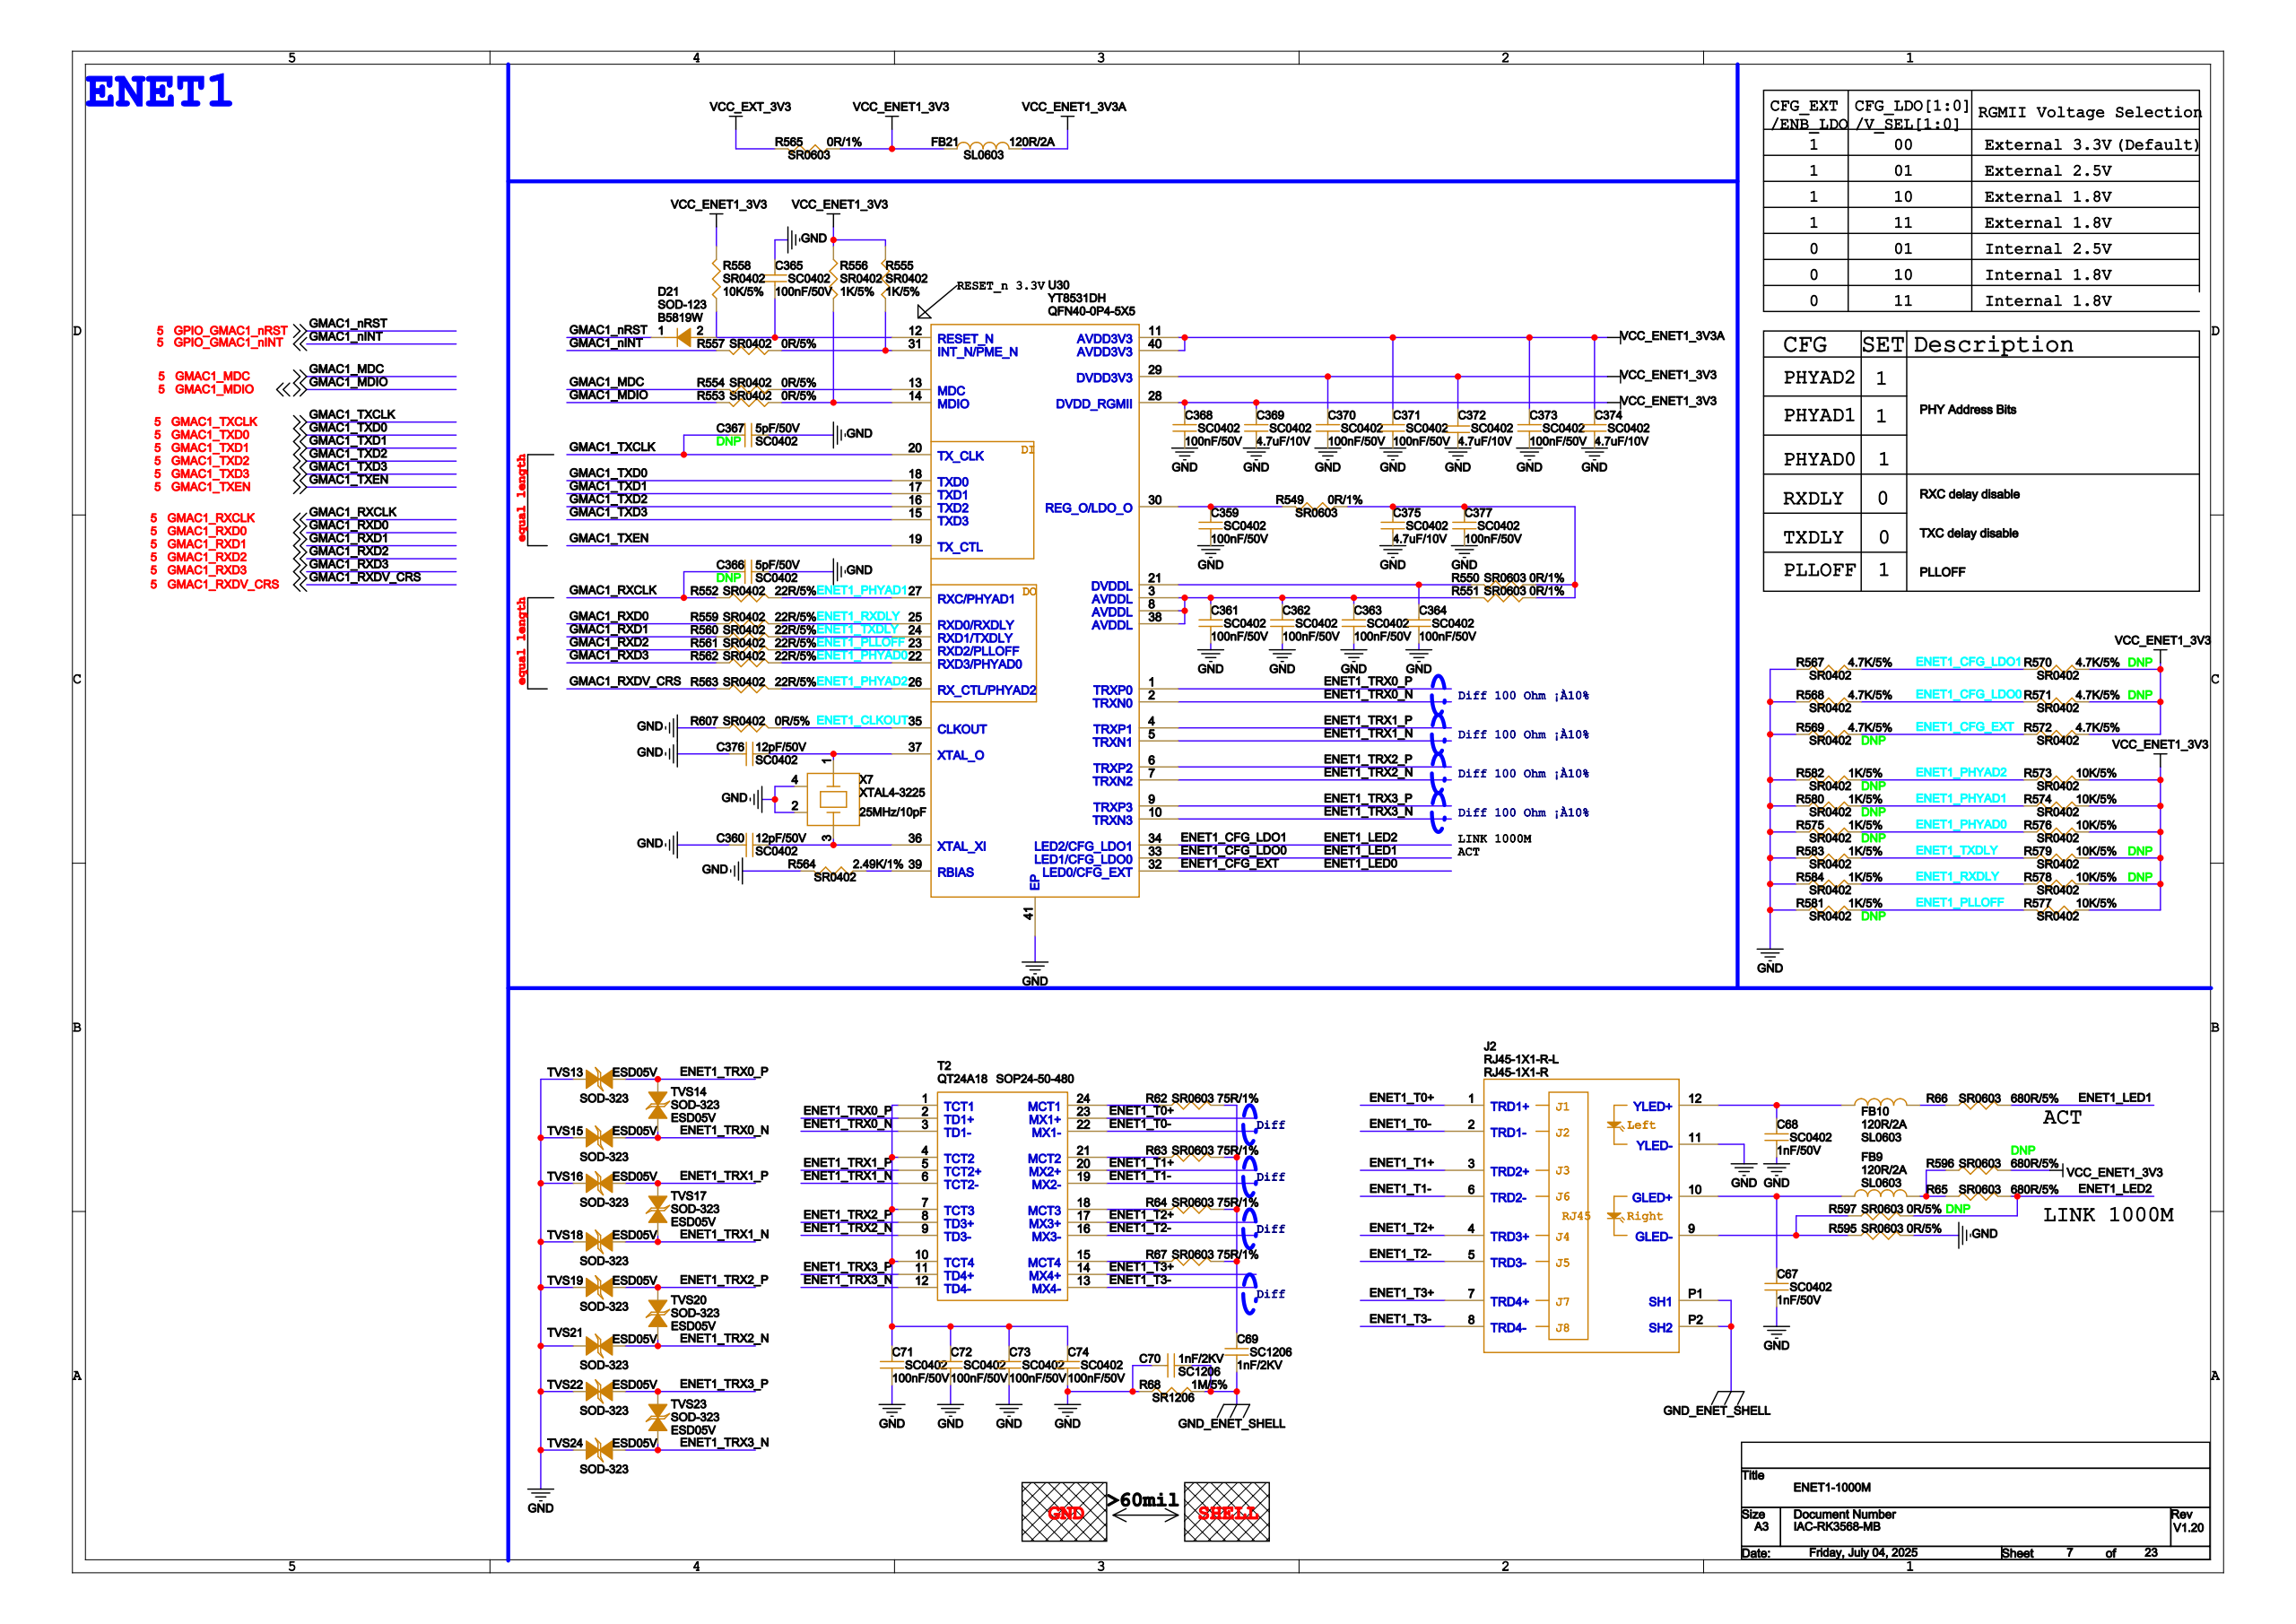Circuit board | Cadence Allegro | 1138 parts | 722 nets | one sheet of the schematic
Parts on this sheet (reference | value | footprint):
C67 | 1nF/50V | SC0402
C68 | 1nF/50V | SC0402
C69 | 1nF/2KV | SC1206
C70 | 1nF/2KV | SC1206
C359 | 100nF/50V | SC0402
C360 | 12pF/50V | SC0402
C361 | 100nF/50V | SC0402
C362 | 100nF/50V | SC0402
C363 | 100nF/50V | SC0402
C364 | 100nF/50V | SC0402
C365 | 100nF/50V | SC0402
C366 | 5pF/50V | SC0402
C367 | 5pF/50V | SC0402
C368 | 100nF/50V | SC0402
C369 | 4.7uF/10V | SC0402
C370 | 100nF/50V | SC0402
C371 | 100nF/50V | SC0402
C372 | 4.7uF/10V | SC0402
C373 | 100nF/50V | SC0402
C374 | 4.7uF/10V | SC0402
C375 | 4.7uF/10V | SC0402
C376 | 12pF/50V | SC0402
C377 | 100nF/50V | SC0402
D21 | B5819W | SOD-123
FB9 | 120R/2A | SL0603
FB10 | 120R/2A | SL0603
FB21 | 120R/2A | SL0603
J2 | RJ45-1X1-R | RJ45-1X1-R-L
J3 | PCIE52-X2-RS | PCIE52-X2-RS-1
J4 | M2-BKEY | M2-BKEY
R62 | 75R/1% | SR0603
R63 | 75R/1% | SR0603
R64 | 75R/1% | SR0603
R65 | 680R/5% | SR0603
R66 | 680R/5% | SR0603
R67 | 75R/1% | SR0603
R68 | 1M/5% | SR1206
R549 | 0R/1% | SR0603
R550 | 0R/1% | SR0603
R551 | 0R/1% | SR0603
R552 | 22R/5% | SR0402
R553 | 0R/5% | SR0402
R554 | 0R/5% | SR0402
R555 | 1K/5% | SR0402
R556 | 1K/5% | SR0402
R557 | 0R/5% | SR0402
R558 | 10K/5% | SR0402
R559 | 22R/5% | SR0402
R560 | 22R/5% | SR0402
R561 | 22R/5% | SR0402
R562 | 22R/5% | SR0402
R563 | 22R/5% | SR0402
R564 | 2.49K/1% | SR0402
R565 | 0R/1% | SR0603
R567 | 4.7K/5% | SR0402
R568 | 4.7K/5% | SR0402
R569 | 4.7K/5% | SR0402
R570 | 4.7K/5% | SR0402
R571 | 4.7K/5% | SR0402
R572 | 4.7K/5% | SR0402
R573 | 10K/5% | SR0402
R574 | 10K/5% | SR0402
R575 | 1K/5% | SR0402
R576 | 10K/5% | SR0402
R577 | 10K/5% | SR0402
R578 | 10K/5% | SR0402
R579 | 10K/5% | SR0402
R580 | 1K/5% | SR0402
R581 | 1K/5% | SR0402
R582 | 1K/5% | SR0402
R583 | 1K/5% | SR0402
R584 | 1K/5% | SR0402
R595 | 0R/5% | SR0603
R596 | 680R/5% | SR0603
R597 | 0R/5% | SR0603
R607 | 0R/5% | SR0402
T2 | QT24A18 | SOP24-50-480
TVS14 | ESD05V | SOD-323
TVS15 | ESD05V | SOD-323
TVS16 | ESD05V | SOD-323
TVS17 | ESD05V | SOD-323
TVS18 | ESD05V | SOD-323
TVS19 | ESD05V | SOD-323
TVS20 | ESD05V | SOD-323
TVS21 | ESD05V | SOD-323
TVS22 | ESD05V | SOD-323
TVS23 | ESD05V | SOD-323
TVS24 | ESD05V | SOD-323
U30 | YT8531DH | QFN40-0P4-5X5
X7 | 25MHz/10pF | XTAL4-3225
Nets of these parts (net: part-pin ...):
N5412908: C365-2 D21-2 R558-1 U30-12
GPIO_GMAC1_NRST: D21-1
VCC_EXT_3V3: R565-2
GND: C67-2 C68-2 C70-1 C359-2 C360-2 C361-2 C362-2 C363-2 C364-2 C365-1 C366-2 C367-2 C368-2 C369-2 C370-2 C371-2 C372-1 C373-2 C374-2 C375-2 C376-2 C377-2 J2-11 R68-1 R564-2 R567-1 R568-1 R569-1 R575-1 R580-1 R581-1 R582-1 R583-1 R584-1 R595-2 R607-1 TVS15-1 TVS16-1 TVS18-1 TVS19-1 TVS21-1 TVS22-1 TVS24-1 X7-2 X7-4 J3-4 J3-9 J3-15 J3-18 J3-21 J3-26 J3-27 J3-29 J3-34 J3-35 J3-37 J3-40 J4-3 J4-5 J4-11 J4-27 J4-33 J4-39 U30-41
ENET1_TRX0_P: TVS14-2 T2-2 U30-1
ENET1_TRX0_N: TVS14-1 TVS15-2 T2-3 U30-2
ENET1_TRX1_P: TVS16-2 TVS17-2 T2-5 U30-4
ENET1_TRX1_N: TVS17-1 TVS18-2 T2-6 U30-5
ENET1_TRX2_P: TVS19-2 TVS20-2 T2-8 U30-6
ENET1_TRX2_N: TVS20-1 TVS21-2 T2-9 U30-7
ENET1_TRX3_P: TVS22-2 TVS23-2 T2-11 U30-9
ENET1_TRX3_N: TVS23-1 TVS24-2 T2-12 U30-10
GND_ENET_SHELL: C69-2 C70-2 J2-P1 J2-P2 R68-2
N5451113: C67-1 FB9-1 J2-10
N88979: J2-9 R595-1 R597-1
ENET1_T0+: J2-1 T2-23
ENET1_T0-: J2-2 T2-22
ENET1_T1+: J2-3 T2-20
ENET1_T1-: J2-6 T2-19
ENET1_T2+: J2-4 T2-17
ENET1_T2-: J2-5 T2-16
ENET1_T3+: J2-7 T2-14
ENET1_T3-: J2-8 T2-13
N89027: C68-1 FB10-1 J2-12
N89177: C69-1 R62-2 R63-2 R64-2 R67-2
GMAC1_RXCLK: C366-1 R552-1
GMAC1_TXCLK: C367-1 U30-20
N89287: FB9-2 R65-1 R596-1
VCC_ENET1_3V3: C368-1 C369-1 C370-1 C372-2 FB21-1 R555-2 R556-1 R558-2 R565-1 R570-2 R571-2 R572-2 R573-2 R574-2 R576-2 R577-1 R578-2 R579-2 R596-2 U30-28 U30-29
ENET1_CFG_LDO1: R65-2 R567-2 R570-1 R597-2 U30-34
N89035: FB10-2 R66-1
ENET1_CFG_LDO0: R66-2 R568-2 R571-1 U30-33
N89173: R62-1 T2-24
N89245: R63-1 T2-21
N89317: R64-1 T2-18
N89389: R67-1 T2-15
GPIO_GMAC1_NINT: R557-2
GMAC1_MDC: R554-2
GMAC1_MDIO: R553-2
GMAC1_RXD0: R559-1
GMAC1_RXD1: R560-1
GMAC1_RXD2: R561-1
GMAC1_RXD3: R562-1
GMAC1_RXDV_CRS: R563-1
GMAC1_TXD0: U30-18
GMAC1_TXD1: U30-17
GMAC1_TXD2: U30-16
GMAC1_TXD3: U30-15
GMAC1_TXEN: U30-19
N5413122: C359-1 R549-2 U30-30
N5413456: C361-1 C362-1 C363-1 R551-2 U30-3 U30-8 U30-38
N5413464: C364-1 R550-2 U30-21
VCC_ENET1_3V3A: C371-1 C373-1 C374-1 FB21-2 U30-11 U30-40
N5413070: C375-1 C377-1 R549-1 R550-1 R551-1
N5412486: C360-1 X7-3 U30-36
N5413842: C376-1 X7-1 U30-37
ENET1_PHYAD1: R552-2 R574-1 R580-2 U30-27
ENET1_RXDLY: R559-2 R578-1 R584-2 U30-25
ENET1_TXDLY: R560-2 R579-1 R583-2 U30-24
ENET1_PLLOFF: R561-2 R577-2 R581-2 U30-23
ENET1_PHYAD0: R562-2 R575-2 R576-1 U30-22
ENET1_PHYAD2: R563-2 R573-1 R582-2 U30-26
ENET1_CLKOUT: R607-2 U30-35
N5412580: R553-1 R556-2 U30-14
N5413082: R554-1 U30-13
N5412672: R555-1 R557-1 U30-31
N5412644: R564-1 U30-39
ENET1_CFG_EXT: R569-2 R572-1 U30-32